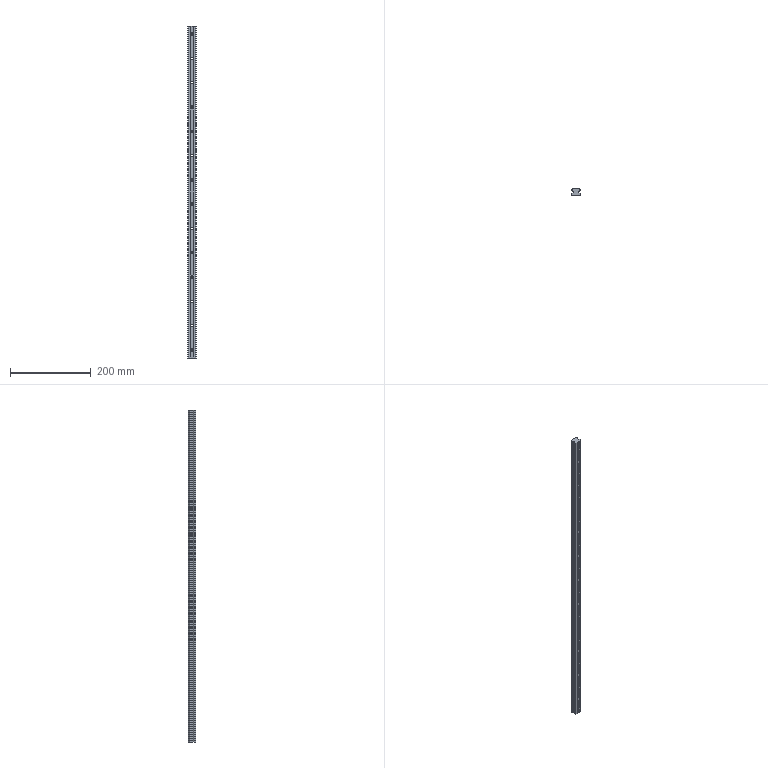Part | SolidWorks | features BaseBody 1 | 1 solid | 142 faces | box 20 x 18 x 820 mm | volume 235286 mm3 | plane 82 | cylinder 60 | commonest cylinder face diameters 6 x28 9.5 x28 4.12 x4